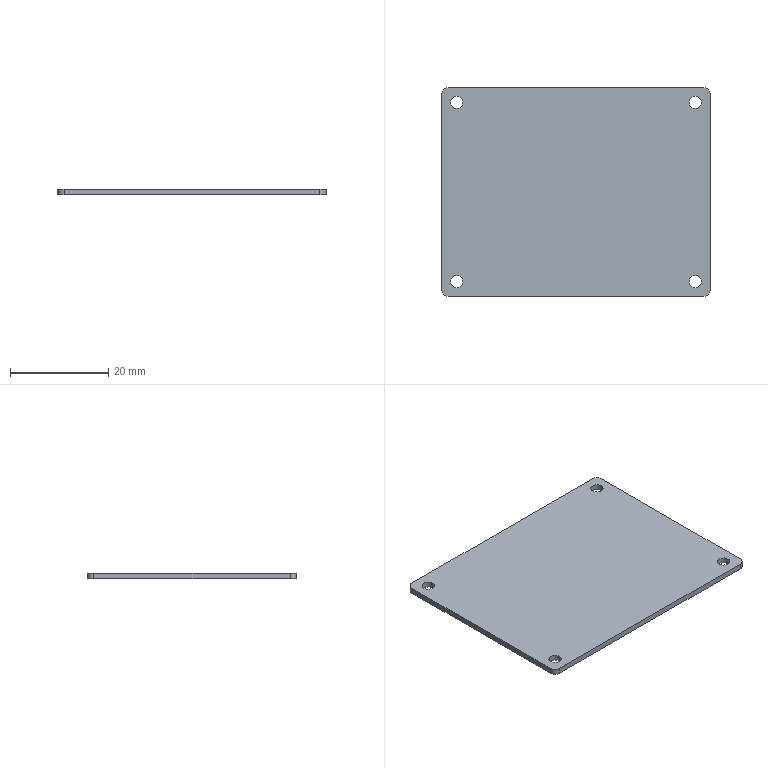Part | STEP file | Control module MCU PCB | 1 solid | 14 faces | box 54.57 x 42.52 x 1.2 mm | volume 2759 mm3 | cylinder 8 | plane 6 | commonest cylinder face diameters 2.5 x4 2.54 x4
STEP:
#1=CARTESIAN_POINT('',(0.,0.,0.));
#2=DIRECTION('',(0.,0.,1.));
#3=DIRECTION('',(1.,0.,0.));
#4=AXIS2_PLACEMENT_3D('',#1,#2,#3);
#5=CARTESIAN_POINT('',(0.209,41.243,0.));
#6=VERTEX_POINT('',#5);
#7=CARTESIAN_POINT('',(0.209,1.263,0.));
#8=VERTEX_POINT('',#7);
#9=CARTESIAN_POINT('',(0.209,41.243,0.));
#10=DIRECTION('',(0.,-1.,0.));
#11=VECTOR('',#10,1.);
#12=LINE('',#9,#11);
#13=CARTESIAN_POINT('',(0.209,41.243,-1.2));
#14=DIRECTION('',(-1.,0.,0.));
#15=DIRECTION('',(0.,0.,1.));
#16=AXIS2_PLACEMENT_3D('',#13,#14,#15);
#17=PLANE('',#16);
#18=CARTESIAN_POINT('',(1.2,0.));
#19=DIRECTION('',(0.,-1.));
#20=VECTOR('',#19,1.);
#21=LINE('',#18,#20);
#22=(GEOMETRIC_REPRESENTATION_CONTEXT(2)PARAMETRIC_REPRESENTATION_CONTEXT()REPRESENTATION_CONTEXT('',''));
#23=DEFINITIONAL_REPRESENTATION('',(#21),#22);
#24=PCURVE('',#17,#23);
#25=CARTESIAN_POINT('',(1.479,1.263,0.));
#26=DIRECTION('',(0.,0.,1.));
#27=DIRECTION('',(1.,0.,0.));
#28=AXIS2_PLACEMENT_3D('',#25,#26,#27);
#29=PLANE('',#28);
#30=CARTESIAN_POINT('',(-1.27,39.98));
#31=DIRECTION('',(0.,-1.));
#32=VECTOR('',#31,1.);
#33=LINE('',#30,#32);
#34=(GEOMETRIC_REPRESENTATION_CONTEXT(2)PARAMETRIC_REPRESENTATION_CONTEXT()REPRESENTATION_CONTEXT('',''));
#35=DEFINITIONAL_REPRESENTATION('',(#33),#34);
#36=PCURVE('',#29,#35);
#37=SURFACE_CURVE('',#12,(#24,#36),.PCURVE_S1.);
#38=EDGE_CURVE('',#6,#8,#37,.T.);
#39=ORIENTED_EDGE('',*,*,#38,.F.);
#40=CARTESIAN_POINT('',(0.209,41.243,-1.2));
#41=VERTEX_POINT('',#40);
#42=CARTESIAN_POINT('',(0.209,41.243,-1.2));
#43=DIRECTION('',(0.,0.,1.));
#44=VECTOR('',#43,1.);
#45=LINE('',#42,#44);
#46=CARTESIAN_POINT('',(0.,0.));
#47=DIRECTION('',(1.,0.));
#48=VECTOR('',#47,1.);
#49=LINE('',#46,#48);
#50=(GEOMETRIC_REPRESENTATION_CONTEXT(2)PARAMETRIC_REPRESENTATION_CONTEXT()REPRESENTATION_CONTEXT('',''));
#51=DEFINITIONAL_REPRESENTATION('',(#49),#50);
#52=PCURVE('',#17,#51);
#53=CARTESIAN_POINT('',(1.479,41.243,-1.2));
#54=DIRECTION('',(0.,0.,1.));
#55=DIRECTION('',(1.,0.,0.));
#56=AXIS2_PLACEMENT_3D('',#53,#54,#55);
#57=CYLINDRICAL_SURFACE('',#56,1.27);
#58=CARTESIAN_POINT('',(3.142,0.));
#59=DIRECTION('',(0.,1.));
#60=VECTOR('',#59,1.);
#61=LINE('',#58,#60);
#62=(GEOMETRIC_REPRESENTATION_CONTEXT(2)PARAMETRIC_REPRESENTATION_CONTEXT()REPRESENTATION_CONTEXT('',''));
#63=DEFINITIONAL_REPRESENTATION('',(#61),#62);
#64=PCURVE('',#57,#63);
#65=SURFACE_CURVE('',#45,(#52,#64),.PCURVE_S1.);
#66=EDGE_CURVE('',#41,#6,#65,.T.);
#67=ORIENTED_EDGE('',*,*,#66,.F.);
#68=CARTESIAN_POINT('',(0.209,1.263,-1.2));
#69=VERTEX_POINT('',#68);
#70=CARTESIAN_POINT('',(0.209,41.243,-1.2));
#71=DIRECTION('',(0.,-1.,0.));
#72=VECTOR('',#71,1.);
#73=LINE('',#70,#72);
#74=CARTESIAN_POINT('',(0.,0.));
#75=DIRECTION('',(0.,-1.));
#76=VECTOR('',#75,1.);
#77=LINE('',#74,#76);
#78=(GEOMETRIC_REPRESENTATION_CONTEXT(2)PARAMETRIC_REPRESENTATION_CONTEXT()REPRESENTATION_CONTEXT('',''));
#79=DEFINITIONAL_REPRESENTATION('',(#77),#78);
#80=PCURVE('',#17,#79);
#81=CARTESIAN_POINT('',(1.479,1.263,-1.2));
#82=DIRECTION('',(0.,0.,1.));
#83=DIRECTION('',(1.,0.,0.));
#84=AXIS2_PLACEMENT_3D('',#81,#82,#83);
#85=PLANE('',#84);
#86=CARTESIAN_POINT('',(-1.27,39.98));
#87=DIRECTION('',(0.,-1.));
#88=VECTOR('',#87,1.);
#89=LINE('',#86,#88);
#90=(GEOMETRIC_REPRESENTATION_CONTEXT(2)PARAMETRIC_REPRESENTATION_CONTEXT()REPRESENTATION_CONTEXT('',''));
#91=DEFINITIONAL_REPRESENTATION('',(#89),#90);
#92=PCURVE('',#85,#91);
#93=SURFACE_CURVE('',#73,(#80,#92),.PCURVE_S1.);
#94=EDGE_CURVE('',#41,#69,#93,.T.);
#95=ORIENTED_EDGE('',*,*,#94,.T.);
#96=CARTESIAN_POINT('',(0.209,1.263,-1.2));
#97=DIRECTION('',(0.,0.,1.));
#98=VECTOR('',#97,1.);
#99=LINE('',#96,#98);
#100=CARTESIAN_POINT('',(0.,-39.98));
#101=DIRECTION('',(1.,0.));
#102=VECTOR('',#101,1.);
#103=LINE('',#100,#102);
#104=(GEOMETRIC_REPRESENTATION_CONTEXT(2)PARAMETRIC_REPRESENTATION_CONTEXT()REPRESENTATION_CONTEXT('',''));
#105=DEFINITIONAL_REPRESENTATION('',(#103),#104);
#106=PCURVE('',#17,#105);
#107=CARTESIAN_POINT('',(1.479,1.263,-1.2));
#108=DIRECTION('',(0.,0.,1.));
#109=DIRECTION('',(1.,0.,0.));
#110=AXIS2_PLACEMENT_3D('',#107,#108,#109);
#111=CYLINDRICAL_SURFACE('',#110,1.27);
#112=CARTESIAN_POINT('',(3.142,0.));
#113=DIRECTION('',(0.,1.));
#114=VECTOR('',#113,1.);
#115=LINE('',#112,#114);
#116=(GEOMETRIC_REPRESENTATION_CONTEXT(2)PARAMETRIC_REPRESENTATION_CONTEXT()REPRESENTATION_CONTEXT('',''));
#117=DEFINITIONAL_REPRESENTATION('',(#115),#116);
#118=PCURVE('',#111,#117);
#119=SURFACE_CURVE('',#99,(#106,#118),.PCURVE_S1.);
#120=EDGE_CURVE('',#69,#8,#119,.T.);
#121=ORIENTED_EDGE('',*,*,#120,.T.);
#122=EDGE_LOOP('',(#39,#67,#95,#121));
#123=FACE_BOUND('',#122,.T.);
#124=ADVANCED_FACE('',(#123),#17,.T.);
#125=CARTESIAN_POINT('',(1.479,-0.007191,0.));
#126=VERTEX_POINT('',#125);
#127=CARTESIAN_POINT('',(1.479,1.263,0.));
#128=DIRECTION('',(0.,0.,1.));
#129=DIRECTION('',(1.,0.,0.));
#130=AXIS2_PLACEMENT_3D('',#127,#128,#129);
#131=CIRCLE('',#130,1.27);
#132=CARTESIAN_POINT('',(0.,1.2));
#133=DIRECTION('',(1.,0.));
#134=VECTOR('',#133,1.);
#135=LINE('',#132,#134);
#136=(GEOMETRIC_REPRESENTATION_CONTEXT(2)PARAMETRIC_REPRESENTATION_CONTEXT()REPRESENTATION_CONTEXT('',''));
#137=DEFINITIONAL_REPRESENTATION('',(#135),#136);
#138=PCURVE('',#111,#137);
#139=CARTESIAN_POINT('',(0.,0.));
#140=DIRECTION('',(1.,0.));
#141=AXIS2_PLACEMENT_2D('',#139,#140);
#142=CIRCLE('',#141,1.27);
#143=(GEOMETRIC_REPRESENTATION_CONTEXT(2)PARAMETRIC_REPRESENTATION_CONTEXT()REPRESENTATION_CONTEXT('',''));
#144=DEFINITIONAL_REPRESENTATION('',(#142),#143);
#145=PCURVE('',#29,#144);
#146=SURFACE_CURVE('',#131,(#138,#145),.PCURVE_S1.);
#147=EDGE_CURVE('',#8,#126,#146,.T.);
#148=ORIENTED_EDGE('',*,*,#147,.F.);
#149=ORIENTED_EDGE('',*,*,#120,.F.);
#150=CARTESIAN_POINT('',(1.479,-0.007191,-1.2));
#151=VERTEX_POINT('',#150);
#152=CARTESIAN_POINT('',(1.479,1.263,-1.2));
#153=DIRECTION('',(0.,0.,1.));
#154=DIRECTION('',(1.,0.,0.));
#155=AXIS2_PLACEMENT_3D('',#152,#153,#154);
#156=CIRCLE('',#155,1.27);
#157=CARTESIAN_POINT('',(0.,0.));
#158=DIRECTION('',(1.,0.));
#159=VECTOR('',#158,1.);
#160=LINE('',#157,#159);
#161=(GEOMETRIC_REPRESENTATION_CONTEXT(2)PARAMETRIC_REPRESENTATION_CONTEXT()REPRESENTATION_CONTEXT('',''));
#162=DEFINITIONAL_REPRESENTATION('',(#160),#161);
#163=PCURVE('',#111,#162);
#164=CARTESIAN_POINT('',(0.,0.));
#165=DIRECTION('',(1.,0.));
#166=AXIS2_PLACEMENT_2D('',#164,#165);
#167=CIRCLE('',#166,1.27);
#168=(GEOMETRIC_REPRESENTATION_CONTEXT(2)PARAMETRIC_REPRESENTATION_CONTEXT()REPRESENTATION_CONTEXT('',''));
#169=DEFINITIONAL_REPRESENTATION('',(#167),#168);
#170=PCURVE('',#85,#169);
#171=SURFACE_CURVE('',#156,(#163,#170),.PCURVE_S1.);
#172=EDGE_CURVE('',#69,#151,#171,.T.);
#173=ORIENTED_EDGE('',*,*,#172,.T.);
#174=CARTESIAN_POINT('',(1.479,-0.007191,-1.2));
#175=DIRECTION('',(0.,0.,1.));
#176=VECTOR('',#175,1.);
#177=LINE('',#174,#176);
#178=CARTESIAN_POINT('',(4.712,0.));
#179=DIRECTION('',(0.,1.));
#180=VECTOR('',#179,1.);
#181=LINE('',#178,#180);
#182=(GEOMETRIC_REPRESENTATION_CONTEXT(2)PARAMETRIC_REPRESENTATION_CONTEXT()REPRESENTATION_CONTEXT('',''));
#183=DEFINITIONAL_REPRESENTATION('',(#181),#182);
#184=PCURVE('',#111,#183);
#185=CARTESIAN_POINT('',(1.479,-0.007191,-1.2));
#186=DIRECTION('',(0.,-1.,0.));
#187=DIRECTION('',(0.,0.,-1.));
#188=AXIS2_PLACEMENT_3D('',#185,#186,#187);
#189=PLANE('',#188);
#190=CARTESIAN_POINT('',(0.,0.));
#191=DIRECTION('',(-1.,0.));
#192=VECTOR('',#191,1.);
#193=LINE('',#190,#192);
#194=(GEOMETRIC_REPRESENTATION_CONTEXT(2)PARAMETRIC_REPRESENTATION_CONTEXT()REPRESENTATION_CONTEXT('',''));
#195=DEFINITIONAL_REPRESENTATION('',(#193),#194);
#196=PCURVE('',#189,#195);
#197=SURFACE_CURVE('',#177,(#184,#196),.PCURVE_S1.);
#198=EDGE_CURVE('',#151,#126,#197,.T.);
#199=ORIENTED_EDGE('',*,*,#198,.T.);
#200=EDGE_LOOP('',(#148,#149,#173,#199));
#201=FACE_BOUND('',#200,.T.);
#202=ADVANCED_FACE('',(#201),#111,.T.);
#203=CARTESIAN_POINT('',(53.509,-0.007191,0.));
#204=VERTEX_POINT('',#203);
#205=CARTESIAN_POINT('',(1.479,-0.007191,0.));
#206=DIRECTION('',(1.,0.,0.));
#207=VECTOR('',#206,1.);
#208=LINE('',#205,#207);
#209=CARTESIAN_POINT('',(-1.2,0.));
#210=DIRECTION('',(0.,1.));
#211=VECTOR('',#210,1.);
#212=LINE('',#209,#211);
#213=(GEOMETRIC_REPRESENTATION_CONTEXT(2)PARAMETRIC_REPRESENTATION_CONTEXT()REPRESENTATION_CONTEXT('',''));
#214=DEFINITIONAL_REPRESENTATION('',(#212),#213);
#215=PCURVE('',#189,#214);
#216=CARTESIAN_POINT('',(0.,-1.27));
#217=DIRECTION('',(1.,0.));
#218=VECTOR('',#217,1.);
#219=LINE('',#216,#218);
#220=(GEOMETRIC_REPRESENTATION_CONTEXT(2)PARAMETRIC_REPRESENTATION_CONTEXT()REPRESENTATION_CONTEXT('',''));
#221=DEFINITIONAL_REPRESENTATION('',(#219),#220);
#222=PCURVE('',#29,#221);
#223=SURFACE_CURVE('',#208,(#215,#222),.PCURVE_S1.);
#224=EDGE_CURVE('',#126,#204,#223,.T.);
#225=ORIENTED_EDGE('',*,*,#224,.F.);
#226=ORIENTED_EDGE('',*,*,#198,.F.);
#227=CARTESIAN_POINT('',(53.509,-0.007191,-1.2));
#228=VERTEX_POINT('',#227);
#229=CARTESIAN_POINT('',(1.479,-0.007191,-1.2));
#230=DIRECTION('',(1.,0.,0.));
#231=VECTOR('',#230,1.);
#232=LINE('',#229,#231);
#233=CARTESIAN_POINT('',(0.,0.));
#234=DIRECTION('',(0.,1.));
#235=VECTOR('',#234,1.);
#236=LINE('',#233,#235);
#237=(GEOMETRIC_REPRESENTATION_CONTEXT(2)PARAMETRIC_REPRESENTATION_CONTEXT()REPRESENTATION_CONTEXT('',''));
#238=DEFINITIONAL_REPRESENTATION('',(#236),#237);
#239=PCURVE('',#189,#238);
#240=CARTESIAN_POINT('',(0.,-1.27));
#241=DIRECTION('',(1.,0.));
#242=VECTOR('',#241,1.);
#243=LINE('',#240,#242);
#244=(GEOMETRIC_REPRESENTATION_CONTEXT(2)PARAMETRIC_REPRESENTATION_CONTEXT()REPRESENTATION_CONTEXT('',''));
#245=DEFINITIONAL_REPRESENTATION('',(#243),#244);
#246=PCURVE('',#85,#245);
#247=SURFACE_CURVE('',#232,(#239,#246),.PCURVE_S1.);
#248=EDGE_CURVE('',#151,#228,#247,.T.);
#249=ORIENTED_EDGE('',*,*,#248,.T.);
#250=CARTESIAN_POINT('',(53.509,-0.007191,-1.2));
#251=DIRECTION('',(0.,0.,1.));
#252=VECTOR('',#251,1.);
#253=LINE('',#250,#252);
#254=CARTESIAN_POINT('',(0.,52.03));
#255=DIRECTION('',(-1.,0.));
#256=VECTOR('',#255,1.);
#257=LINE('',#254,#256);
#258=(GEOMETRIC_REPRESENTATION_CONTEXT(2)PARAMETRIC_REPRESENTATION_CONTEXT()REPRESENTATION_CONTEXT('',''));
#259=DEFINITIONAL_REPRESENTATION('',(#257),#258);
#260=PCURVE('',#189,#259);
#261=CARTESIAN_POINT('',(53.509,1.263,-1.2));
#262=DIRECTION('',(0.,0.,1.));
#263=DIRECTION('',(1.,0.,0.));
#264=AXIS2_PLACEMENT_3D('',#261,#262,#263);
#265=CYLINDRICAL_SURFACE('',#264,1.27);
#266=CARTESIAN_POINT('',(4.712,0.));
#267=DIRECTION('',(0.,1.));
#268=VECTOR('',#267,1.);
#269=LINE('',#266,#268);
#270=(GEOMETRIC_REPRESENTATION_CONTEXT(2)PARAMETRIC_REPRESENTATION_CONTEXT()REPRESENTATION_CONTEXT('',''));
#271=DEFINITIONAL_REPRESENTATION('',(#269),#270);
#272=PCURVE('',#265,#271);
#273=SURFACE_CURVE('',#253,(#260,#272),.PCURVE_S1.);
#274=EDGE_CURVE('',#228,#204,#273,.T.);
#275=ORIENTED_EDGE('',*,*,#274,.T.);
#276=EDGE_LOOP('',(#225,#226,#249,#275));
#277=FACE_BOUND('',#276,.T.);
#278=ADVANCED_FACE('',(#277),#189,.T.);
#279=CARTESIAN_POINT('',(54.779,1.263,0.));
#280=VERTEX_POINT('',#279);
#281=CARTESIAN_POINT('',(53.509,1.263,0.));
#282=DIRECTION('',(0.,0.,1.));
#283=DIRECTION('',(1.,0.,0.));
#284=AXIS2_PLACEMENT_3D('',#281,#282,#283);
#285=CIRCLE('',#284,1.27);
#286=CARTESIAN_POINT('',(0.,1.2));
#287=DIRECTION('',(1.,0.));
#288=VECTOR('',#287,1.);
#289=LINE('',#286,#288);
#290=(GEOMETRIC_REPRESENTATION_CONTEXT(2)PARAMETRIC_REPRESENTATION_CONTEXT()REPRESENTATION_CONTEXT('',''));
#291=DEFINITIONAL_REPRESENTATION('',(#289),#290);
#292=PCURVE('',#265,#291);
#293=CARTESIAN_POINT('',(52.03,0.));
#294=DIRECTION('',(1.,0.));
#295=AXIS2_PLACEMENT_2D('',#293,#294);
#296=CIRCLE('',#295,1.27);
#297=(GEOMETRIC_REPRESENTATION_CONTEXT(2)PARAMETRIC_REPRESENTATION_CONTEXT()REPRESENTATION_CONTEXT('',''));
#298=DEFINITIONAL_REPRESENTATION('',(#296),#297);
#299=PCURVE('',#29,#298);
#300=SURFACE_CURVE('',#285,(#292,#299),.PCURVE_S1.);
#301=EDGE_CURVE('',#204,#280,#300,.T.);
#302=ORIENTED_EDGE('',*,*,#301,.F.);
#303=ORIENTED_EDGE('',*,*,#274,.F.);
#304=CARTESIAN_POINT('',(54.779,1.263,-1.2));
#305=VERTEX_POINT('',#304);
#306=CARTESIAN_POINT('',(53.509,1.263,-1.2));
#307=DIRECTION('',(0.,0.,1.));
#308=DIRECTION('',(1.,0.,0.));
#309=AXIS2_PLACEMENT_3D('',#306,#307,#308);
#310=CIRCLE('',#309,1.27);
#311=CARTESIAN_POINT('',(0.,0.));
#312=DIRECTION('',(1.,0.));
#313=VECTOR('',#312,1.);
#314=LINE('',#311,#313);
#315=(GEOMETRIC_REPRESENTATION_CONTEXT(2)PARAMETRIC_REPRESENTATION_CONTEXT()REPRESENTATION_CONTEXT('',''));
#316=DEFINITIONAL_REPRESENTATION('',(#314),#315);
#317=PCURVE('',#265,#316);
#318=CARTESIAN_POINT('',(52.03,0.));
#319=DIRECTION('',(1.,0.));
#320=AXIS2_PLACEMENT_2D('',#318,#319);
#321=CIRCLE('',#320,1.27);
#322=(GEOMETRIC_REPRESENTATION_CONTEXT(2)PARAMETRIC_REPRESENTATION_CONTEXT()REPRESENTATION_CONTEXT('',''));
#323=DEFINITIONAL_REPRESENTATION('',(#321),#322);
#324=PCURVE('',#85,#323);
#325=SURFACE_CURVE('',#310,(#317,#324),.PCURVE_S1.);
#326=EDGE_CURVE('',#228,#305,#325,.T.);
#327=ORIENTED_EDGE('',*,*,#326,.T.);
#328=CARTESIAN_POINT('',(54.779,1.263,-1.2));
#329=DIRECTION('',(0.,0.,1.));
#330=VECTOR('',#329,1.);
#331=LINE('',#328,#330);
#332=CARTESIAN_POINT('',(6.283,0.));
#333=DIRECTION('',(0.,1.));
#334=VECTOR('',#333,1.);
#335=LINE('',#332,#334);
#336=(GEOMETRIC_REPRESENTATION_CONTEXT(2)PARAMETRIC_REPRESENTATION_CONTEXT()REPRESENTATION_CONTEXT('',''));
#337=DEFINITIONAL_REPRESENTATION('',(#335),#336);
#338=PCURVE('',#265,#337);
#339=CARTESIAN_POINT('',(54.779,1.263,-1.2));
#340=DIRECTION('',(1.,0.000000064,0.));
#341=DIRECTION('',(-0.000000064,1.,0.));
#342=AXIS2_PLACEMENT_3D('',#339,#340,#341);
#343=PLANE('',#342);
#344=CARTESIAN_POINT('',(0.,0.));
#345=DIRECTION('',(0.,1.));
#346=VECTOR('',#345,1.);
#347=LINE('',#344,#346);
#348=(GEOMETRIC_REPRESENTATION_CONTEXT(2)PARAMETRIC_REPRESENTATION_CONTEXT()REPRESENTATION_CONTEXT('',''));
#349=DEFINITIONAL_REPRESENTATION('',(#347),#348);
#350=PCURVE('',#343,#349);
#351=SURFACE_CURVE('',#331,(#338,#350),.PCURVE_S1.);
#352=EDGE_CURVE('',#305,#280,#351,.T.);
#353=ORIENTED_EDGE('',*,*,#352,.T.);
#354=EDGE_LOOP('',(#302,#303,#327,#353));
#355=FACE_BOUND('',#354,.T.);
#356=ADVANCED_FACE('',(#355),#265,.T.);
#357=CARTESIAN_POINT('',(54.779,41.243,0.));
#358=VERTEX_POINT('',#357);
#359=CARTESIAN_POINT('',(54.779,1.263,0.));
#360=DIRECTION('',(-0.000000064,1.,0.));
#361=VECTOR('',#360,1.);
#362=LINE('',#359,#361);
#363=CARTESIAN_POINT('',(0.,1.2));
#364=DIRECTION('',(1.,0.));
#365=VECTOR('',#364,1.);
#366=LINE('',#363,#365);
#367=(GEOMETRIC_REPRESENTATION_CONTEXT(2)PARAMETRIC_REPRESENTATION_CONTEXT()REPRESENTATION_CONTEXT('',''));
#368=DEFINITIONAL_REPRESENTATION('',(#366),#367);
#369=PCURVE('',#343,#368);
#370=CARTESIAN_POINT('',(53.3,0.));
#371=DIRECTION('',(-0.000000064,1.));
#372=VECTOR('',#371,1.);
#373=LINE('',#370,#372);
#374=(GEOMETRIC_REPRESENTATION_CONTEXT(2)PARAMETRIC_REPRESENTATION_CONTEXT()REPRESENTATION_CONTEXT('',''));
#375=DEFINITIONAL_REPRESENTATION('',(#373),#374);
#376=PCURVE('',#29,#375);
#377=SURFACE_CURVE('',#362,(#369,#376),.PCURVE_S1.);
#378=EDGE_CURVE('',#280,#358,#377,.T.);
#379=ORIENTED_EDGE('',*,*,#378,.F.);
#380=ORIENTED_EDGE('',*,*,#352,.F.);
#381=CARTESIAN_POINT('',(54.779,41.243,-1.2));
#382=VERTEX_POINT('',#381);
#383=CARTESIAN_POINT('',(54.779,1.263,-1.2));
#384=DIRECTION('',(-0.000000064,1.,0.));
#385=VECTOR('',#384,1.);
#386=LINE('',#383,#385);
#387=CARTESIAN_POINT('',(0.,0.));
#388=DIRECTION('',(1.,0.));
#389=VECTOR('',#388,1.);
#390=LINE('',#387,#389);
#391=(GEOMETRIC_REPRESENTATION_CONTEXT(2)PARAMETRIC_REPRESENTATION_CONTEXT()REPRESENTATION_CONTEXT('',''));
#392=DEFINITIONAL_REPRESENTATION('',(#390),#391);
#393=PCURVE('',#343,#392);
#394=CARTESIAN_POINT('',(53.3,0.));
#395=DIRECTION('',(-0.000000064,1.));
#396=VECTOR('',#395,1.);
#397=LINE('',#394,#396);
#398=(GEOMETRIC_REPRESENTATION_CONTEXT(2)PARAMETRIC_REPRESENTATION_CONTEXT()REPRESENTATION_CONTEXT('',''));
#399=DEFINITIONAL_REPRESENTATION('',(#397),#398);
#400=PCURVE('',#85,#399);
#401=SURFACE_CURVE('',#386,(#393,#400),.PCURVE_S1.);
#402=EDGE_CURVE('',#305,#382,#401,.T.);
#403=ORIENTED_EDGE('',*,*,#402,.T.);
#404=CARTESIAN_POINT('',(54.779,41.243,-1.2));
#405=DIRECTION('',(0.,0.,1.));
#406=VECTOR('',#405,1.);
#407=LINE('',#404,#406);
#408=CARTESIAN_POINT('',(39.98,0.));
#409=DIRECTION('',(0.,1.));
#410=VECTOR('',#409,1.);
#411=LINE('',#408,#410);
#412=(GEOMETRIC_REPRESENTATION_CONTEXT(2)PARAMETRIC_REPRESENTATION_CONTEXT()REPRESENTATION_CONTEXT('',''));
#413=DEFINITIONAL_REPRESENTATION('',(#411),#412);
#414=PCURVE('',#343,#413);
#415=CARTESIAN_POINT('',(53.509,41.243,-1.2));
#416=DIRECTION('',(0.,0.,1.));
#417=DIRECTION('',(1.,0.,0.));
#418=AXIS2_PLACEMENT_3D('',#415,#416,#417);
#419=CYLINDRICAL_SURFACE('',#418,1.27);
#420=CARTESIAN_POINT('',(0.,0.));
#421=DIRECTION('',(0.,1.));
#422=VECTOR('',#421,1.);
#423=LINE('',#420,#422);
#424=(GEOMETRIC_REPRESENTATION_CONTEXT(2)PARAMETRIC_REPRESENTATION_CONTEXT()REPRESENTATION_CONTEXT('',''));
#425=DEFINITIONAL_REPRESENTATION('',(#423),#424);
#426=PCURVE('',#419,#425);
#427=SURFACE_CURVE('',#407,(#414,#426),.PCURVE_S1.);
#428=EDGE_CURVE('',#382,#358,#427,.T.);
#429=ORIENTED_EDGE('',*,*,#428,.T.);
#430=EDGE_LOOP('',(#379,#380,#403,#429));
#431=FACE_BOUND('',#430,.T.);
#432=ADVANCED_FACE('',(#431),#343,.T.);
#433=CARTESIAN_POINT('',(53.509,42.513,0.));
#434=VERTEX_POINT('',#433);
#435=CARTESIAN_POINT('',(53.509,41.243,0.));
#436=DIRECTION('',(0.,0.,1.));
#437=DIRECTION('',(1.,0.,0.));
#438=AXIS2_PLACEMENT_3D('',#435,#436,#437);
#439=CIRCLE('',#438,1.27);
#440=CARTESIAN_POINT('',(0.,1.2));
#441=DIRECTION('',(1.,0.));
#442=VECTOR('',#441,1.);
#443=LINE('',#440,#442);
#444=(GEOMETRIC_REPRESENTATION_CONTEXT(2)PARAMETRIC_REPRESENTATION_CONTEXT()REPRESENTATION_CONTEXT('',''));
#445=DEFINITIONAL_REPRESENTATION('',(#443),#444);
#446=PCURVE('',#419,#445);
#447=CARTESIAN_POINT('',(52.03,39.98));
#448=DIRECTION('',(1.,0.));
#449=AXIS2_PLACEMENT_2D('',#447,#448);
#450=CIRCLE('',#449,1.27);
#451=(GEOMETRIC_REPRESENTATION_CONTEXT(2)PARAMETRIC_REPRESENTATION_CONTEXT()REPRESENTATION_CONTEXT('',''));
#452=DEFINITIONAL_REPRESENTATION('',(#450),#451);
#453=PCURVE('',#29,#452);
#454=SURFACE_CURVE('',#439,(#446,#453),.PCURVE_S1.);
#455=EDGE_CURVE('',#358,#434,#454,.T.);
#456=ORIENTED_EDGE('',*,*,#455,.F.);
#457=ORIENTED_EDGE('',*,*,#428,.F.);
#458=CARTESIAN_POINT('',(53.509,42.513,-1.2));
#459=VERTEX_POINT('',#458);
#460=CARTESIAN_POINT('',(53.509,41.243,-1.2));
#461=DIRECTION('',(0.,0.,1.));
#462=DIRECTION('',(1.,0.,0.));
#463=AXIS2_PLACEMENT_3D('',#460,#461,#462);
#464=CIRCLE('',#463,1.27);
#465=CARTESIAN_POINT('',(0.,0.));
#466=DIRECTION('',(1.,0.));
#467=VECTOR('',#466,1.);
#468=LINE('',#465,#467);
#469=(GEOMETRIC_REPRESENTATION_CONTEXT(2)PARAMETRIC_REPRESENTATION_CONTEXT()REPRESENTATION_CONTEXT('',''));
#470=DEFINITIONAL_REPRESENTATION('',(#468),#469);
#471=PCURVE('',#419,#470);
#472=CARTESIAN_POINT('',(52.03,39.98));
#473=DIRECTION('',(1.,0.));
#474=AXIS2_PLACEMENT_2D('',#472,#473);
#475=CIRCLE('',#474,1.27);
#476=(GEOMETRIC_REPRESENTATION_CONTEXT(2)PARAMETRIC_REPRESENTATION_CONTEXT()REPRESENTATION_CONTEXT('',''));
#477=DEFINITIONAL_REPRESENTATION('',(#475),#476);
#478=PCURVE('',#85,#477);
#479=SURFACE_CURVE('',#464,(#471,#478),.PCURVE_S1.);
#480=EDGE_CURVE('',#382,#459,#479,.T.);
#481=ORIENTED_EDGE('',*,*,#480,.T.);
#482=CARTESIAN_POINT('',(53.509,42.513,-1.2));
#483=DIRECTION('',(0.,0.,1.));
#484=VECTOR('',#483,1.);
#485=LINE('',#482,#484);
#486=CARTESIAN_POINT('',(1.571,0.));
#487=DIRECTION('',(0.,1.));
#488=VECTOR('',#487,1.);
#489=LINE('',#486,#488);
#490=(GEOMETRIC_REPRESENTATION_CONTEXT(2)PARAMETRIC_REPRESENTATION_CONTEXT()REPRESENTATION_CONTEXT('',''));
#491=DEFINITIONAL_REPRESENTATION('',(#489),#490);
#492=PCURVE('',#419,#491);
#493=CARTESIAN_POINT('',(53.509,42.513,-1.2));
#494=DIRECTION('',(0.,1.,0.));
#495=DIRECTION('',(0.,0.,1.));
#496=AXIS2_PLACEMENT_3D('',#493,#494,#495);
#497=PLANE('',#496);
#498=CARTESIAN_POINT('',(0.,0.));
#499=DIRECTION('',(1.,0.));
#500=VECTOR('',#499,1.);
#501=LINE('',#498,#500);
#502=(GEOMETRIC_REPRESENTATION_CONTEXT(2)PARAMETRIC_REPRESENTATION_CONTEXT()REPRESENTATION_CONTEXT('',''));
#503=DEFINITIONAL_REPRESENTATION('',(#501),#502);
#504=PCURVE('',#497,#503);
#505=SURFACE_CURVE('',#485,(#492,#504),.PCURVE_S1.);
#506=EDGE_CURVE('',#459,#434,#505,.T.);
#507=ORIENTED_EDGE('',*,*,#506,.T.);
#508=EDGE_LOOP('',(#456,#457,#481,#507));
#509=FACE_BOUND('',#508,.T.);
#510=ADVANCED_FACE('',(#509),#419,.T.);
#511=CARTESIAN_POINT('',(1.479,42.513,0.));
#512=VERTEX_POINT('',#511);
#513=CARTESIAN_POINT('',(53.509,42.513,0.));
#514=DIRECTION('',(-1.,0.,0.));
#515=VECTOR('',#514,1.);
#516=LINE('',#513,#515);
#517=CARTESIAN_POINT('',(1.2,0.));
#518=DIRECTION('',(0.,-1.));
#519=VECTOR('',#518,1.);
#520=LINE('',#517,#519);
#521=(GEOMETRIC_REPRESENTATION_CONTEXT(2)PARAMETRIC_REPRESENTATION_CONTEXT()REPRESENTATION_CONTEXT('',''));
#522=DEFINITIONAL_REPRESENTATION('',(#520),#521);
#523=PCURVE('',#497,#522);
#524=CARTESIAN_POINT('',(52.03,41.25));
#525=DIRECTION('',(-1.,0.));
#526=VECTOR('',#525,1.);
#527=LINE('',#524,#526);
#528=(GEOMETRIC_REPRESENTATION_CONTEXT(2)PARAMETRIC_REPRESENTATION_CONTEXT()REPRESENTATION_CONTEXT('',''));
#529=DEFINITIONAL_REPRESENTATION('',(#527),#528);
#530=PCURVE('',#29,#529);
#531=SURFACE_CURVE('',#516,(#523,#530),.PCURVE_S1.);
#532=EDGE_CURVE('',#434,#512,#531,.T.);
#533=ORIENTED_EDGE('',*,*,#532,.F.);
#534=ORIENTED_EDGE('',*,*,#506,.F.);
#535=CARTESIAN_POINT('',(1.479,42.513,-1.2));
#536=VERTEX_POINT('',#535);
#537=CARTESIAN_POINT('',(53.509,42.513,-1.2));
#538=DIRECTION('',(-1.,0.,0.));
#539=VECTOR('',#538,1.);
#540=LINE('',#537,#539);
#541=CARTESIAN_POINT('',(0.,0.));
#542=DIRECTION('',(0.,-1.));
#543=VECTOR('',#542,1.);
#544=LINE('',#541,#543);
#545=(GEOMETRIC_REPRESENTATION_CONTEXT(2)PARAMETRIC_REPRESENTATION_CONTEXT()REPRESENTATION_CONTEXT('',''));
#546=DEFINITIONAL_REPRESENTATION('',(#544),#545);
#547=PCURVE('',#497,#546);
#548=CARTESIAN_POINT('',(52.03,41.25));
#549=DIRECTION('',(-1.,0.));
#550=VECTOR('',#549,1.);
#551=LINE('',#548,#550);
#552=(GEOMETRIC_REPRESENTATION_CONTEXT(2)PARAMETRIC_REPRESENTATION_CONTEXT()REPRESENTATION_CONTEXT('',''));
#553=DEFINITIONAL_REPRESENTATION('',(#551),#552);
#554=PCURVE('',#85,#553);
#555=SURFACE_CURVE('',#540,(#547,#554),.PCURVE_S1.);
#556=EDGE_CURVE('',#459,#536,#555,.T.);
#557=ORIENTED_EDGE('',*,*,#556,.T.);
#558=CARTESIAN_POINT('',(1.479,42.513,-1.2));
#559=DIRECTION('',(0.,0.,1.));
#560=VECTOR('',#559,1.);
#561=LINE('',#558,#560);
#562=CARTESIAN_POINT('',(0.,-52.03));
#563=DIRECTION('',(1.,0.));
#564=VECTOR('',#563,1.);
#565=LINE('',#562,#564);
#566=(GEOMETRIC_REPRESENTATION_CONTEXT(2)PARAMETRIC_REPRESENTATION_CONTEXT()REPRESENTATION_CONTEXT('',''));
#567=DEFINITIONAL_REPRESENTATION('',(#565),#566);
#568=PCURVE('',#497,#567);
#569=CARTESIAN_POINT('',(1.571,0.));
#570=DIRECTION('',(0.,1.));
#571=VECTOR('',#570,1.);
#572=LINE('',#569,#571);
#573=(GEOMETRIC_REPRESENTATION_CONTEXT(2)PARAMETRIC_REPRESENTATION_CONTEXT()REPRESENTATION_CONTEXT('',''));
#574=DEFINITIONAL_REPRESENTATION('',(#572),#573);
#575=PCURVE('',#57,#574);
#576=SURFACE_CURVE('',#561,(#568,#575),.PCURVE_S1.);
#577=EDGE_CURVE('',#536,#512,#576,.T.);
#578=ORIENTED_EDGE('',*,*,#577,.T.);
#579=EDGE_LOOP('',(#533,#534,#557,#578));
#580=FACE_BOUND('',#579,.T.);
#581=ADVANCED_FACE('',(#580),#497,.T.);
#582=CARTESIAN_POINT('',(53.029,2.993,-1.2));
#583=VERTEX_POINT('',#582);
#584=CARTESIAN_POINT('',(51.779,2.993,-1.2));
#585=DIRECTION('',(0.,0.,1.));
#586=DIRECTION('',(1.,0.,0.));
#587=AXIS2_PLACEMENT_3D('',#584,#585,#586);
#588=CIRCLE('',#587,1.25);
#589=CARTESIAN_POINT('',(51.779,2.993,-1.2));
#590=DIRECTION('',(0.,0.,1.));
#591=DIRECTION('',(1.,0.,0.));
#592=AXIS2_PLACEMENT_3D('',#589,#590,#591);
#593=CYLINDRICAL_SURFACE('',#592,1.25);
#594=CARTESIAN_POINT('',(0.,0.));
#595=DIRECTION('',(1.,0.));
#596=VECTOR('',#595,1.);
#597=LINE('',#594,#596);
#598=(GEOMETRIC_REPRESENTATION_CONTEXT(2)PARAMETRIC_REPRESENTATION_CONTEXT()REPRESENTATION_CONTEXT('',''));
#599=DEFINITIONAL_REPRESENTATION('',(#597),#598);
#600=PCURVE('',#593,#599);
#601=CARTESIAN_POINT('',(50.3,1.73));
#602=DIRECTION('',(1.,0.));
#603=AXIS2_PLACEMENT_2D('',#601,#602);
#604=CIRCLE('',#603,1.25);
#605=(GEOMETRIC_REPRESENTATION_CONTEXT(2)PARAMETRIC_REPRESENTATION_CONTEXT()REPRESENTATION_CONTEXT('',''));
#606=DEFINITIONAL_REPRESENTATION('',(#604),#605);
#607=PCURVE('',#85,#606);
#608=SURFACE_CURVE('',#588,(#600,#607),.PCURVE_S1.);
#609=EDGE_CURVE('',#583,#583,#608,.T.);
#610=ORIENTED_EDGE('',*,*,#609,.T.);
#611=CARTESIAN_POINT('',(53.029,2.993,0.));
#612=VERTEX_POINT('',#611);
#613=CARTESIAN_POINT('',(53.029,2.993,-1.2));
#614=CARTESIAN_POINT('',(53.029,2.993,0.));
#615=B_SPLINE_CURVE_WITH_KNOTS('',1,(#613,#614),.UNSPECIFIED.,.F.,.F.,(2,2),(0.,1.2),.PIECEWISE_BEZIER_KNOTS.);
#616=CARTESIAN_POINT('',(6.283,0.));
#617=DIRECTION('',(0.,1.));
#618=VECTOR('',#617,1.);
#619=LINE('',#616,#618);
#620=(GEOMETRIC_REPRESENTATION_CONTEXT(2)PARAMETRIC_REPRESENTATION_CONTEXT()REPRESENTATION_CONTEXT('',''));
#621=DEFINITIONAL_REPRESENTATION('',(#619),#620);
#622=PCURVE('',#593,#621);
#623=CARTESIAN_POINT('',(0.,0.));
#624=DIRECTION('',(0.,1.));
#625=VECTOR('',#624,1.);
#626=LINE('',#623,#625);
#627=(GEOMETRIC_REPRESENTATION_CONTEXT(2)PARAMETRIC_REPRESENTATION_CONTEXT()REPRESENTATION_CONTEXT('',''));
#628=DEFINITIONAL_REPRESENTATION('',(#626),#627);
#629=PCURVE('',#593,#628);
#630=SEAM_CURVE('',#615,(#622,#629),.PCURVE_S1.);
#631=EDGE_CURVE('',#583,#612,#630,.T.);
#632=ORIENTED_EDGE('',*,*,#631,.T.);
#633=CARTESIAN_POINT('',(51.779,2.993,0.));
#634=DIRECTION('',(0.,0.,1.));
#635=DIRECTION('',(1.,0.,0.));
#636=AXIS2_PLACEMENT_3D('',#633,#634,#635);
#637=CIRCLE('',#636,1.25);
#638=CARTESIAN_POINT('',(0.,1.2));
#639=DIRECTION('',(1.,0.));
#640=VECTOR('',#639,1.);
#641=LINE('',#638,#640);
#642=(GEOMETRIC_REPRESENTATION_CONTEXT(2)PARAMETRIC_REPRESENTATION_CONTEXT()REPRESENTATION_CONTEXT('',''));
#643=DEFINITIONAL_REPRESENTATION('',(#641),#642);
#644=PCURVE('',#593,#643);
#645=CARTESIAN_POINT('',(50.3,1.73));
#646=DIRECTION('',(1.,0.));
#647=AXIS2_PLACEMENT_2D('',#645,#646);
#648=CIRCLE('',#647,1.25);
#649=(GEOMETRIC_REPRESENTATION_CONTEXT(2)PARAMETRIC_REPRESENTATION_CONTEXT()REPRESENTATION_CONTEXT('',''));
#650=DEFINITIONAL_REPRESENTATION('',(#648),#649);
#651=PCURVE('',#29,#650);
#652=SURFACE_CURVE('',#637,(#644,#651),.PCURVE_S1.);
#653=EDGE_CURVE('',#612,#612,#652,.T.);
#654=ORIENTED_EDGE('',*,*,#653,.F.);
#655=ORIENTED_EDGE('',*,*,#631,.F.);
#656=EDGE_LOOP('',(#610,#632,#654,#655));
#657=FACE_BOUND('',#656,.F.);
#658=ADVANCED_FACE('',(#657),#593,.F.);
#659=CARTESIAN_POINT('',(4.459,2.993,-1.2));
#660=VERTEX_POINT('',#659);
#661=CARTESIAN_POINT('',(3.209,2.993,-1.2));
#662=DIRECTION('',(0.,0.,1.));
#663=DIRECTION('',(1.,0.,0.));
#664=AXIS2_PLACEMENT_3D('',#661,#662,#663);
#665=CIRCLE('',#664,1.25);
#666=CARTESIAN_POINT('',(3.209,2.993,-1.2));
#667=DIRECTION('',(0.,0.,1.));
#668=DIRECTION('',(1.,0.,0.));
#669=AXIS2_PLACEMENT_3D('',#666,#667,#668);
#670=CYLINDRICAL_SURFACE('',#669,1.25);
#671=CARTESIAN_POINT('',(0.,0.));
#672=DIRECTION('',(1.,0.));
#673=VECTOR('',#672,1.);
#674=LINE('',#671,#673);
#675=(GEOMETRIC_REPRESENTATION_CONTEXT(2)PARAMETRIC_REPRESENTATION_CONTEXT()REPRESENTATION_CONTEXT('',''));
#676=DEFINITIONAL_REPRESENTATION('',(#674),#675);
#677=PCURVE('',#670,#676);
#678=CARTESIAN_POINT('',(1.73,1.73));
#679=DIRECTION('',(1.,0.));
#680=AXIS2_PLACEMENT_2D('',#678,#679);
#681=CIRCLE('',#680,1.25);
#682=(GEOMETRIC_REPRESENTATION_CONTEXT(2)PARAMETRIC_REPRESENTATION_CONTEXT()REPRESENTATION_CONTEXT('',''));
#683=DEFINITIONAL_REPRESENTATION('',(#681),#682);
#684=PCURVE('',#85,#683);
#685=SURFACE_CURVE('',#665,(#677,#684),.PCURVE_S1.);
#686=EDGE_CURVE('',#660,#660,#685,.T.);
#687=ORIENTED_EDGE('',*,*,#686,.T.);
#688=CARTESIAN_POINT('',(4.459,2.993,0.));
#689=VERTEX_POINT('',#688);
#690=CARTESIAN_POINT('',(4.459,2.993,-1.2));
#691=CARTESIAN_POINT('',(4.459,2.993,0.));
#692=B_SPLINE_CURVE_WITH_KNOTS('',1,(#690,#691),.UNSPECIFIED.,.F.,.F.,(2,2),(0.,1.2),.PIECEWISE_BEZIER_KNOTS.);
#693=CARTESIAN_POINT('',(6.283,0.));
#694=DIRECTION('',(0.,1.));
#695=VECTOR('',#694,1.);
#696=LINE('',#693,#695);
#697=(GEOMETRIC_REPRESENTATION_CONTEXT(2)PARAMETRIC_REPRESENTATION_CONTEXT()REPRESENTATION_CONTEXT('',''));
#698=DEFINITIONAL_REPRESENTATION('',(#696),#697);
#699=PCURVE('',#670,#698);
#700=CARTESIAN_POINT('',(0.,0.));
#701=DIRECTION('',(0.,1.));
#702=VECTOR('',#701,1.);
#703=LINE('',#700,#702);
#704=(GEOMETRIC_REPRESENTATION_CONTEXT(2)PARAMETRIC_REPRESENTATION_CONTEXT()REPRESENTATION_CONTEXT('',''));
#705=DEFINITIONAL_REPRESENTATION('',(#703),#704);
#706=PCURVE('',#670,#705);
#707=SEAM_CURVE('',#692,(#699,#706),.PCURVE_S1.);
#708=EDGE_CURVE('',#660,#689,#707,.T.);
#709=ORIENTED_EDGE('',*,*,#708,.T.);
#710=CARTESIAN_POINT('',(3.209,2.993,0.));
#711=DIRECTION('',(0.,0.,1.));
#712=DIRECTION('',(1.,0.,0.));
#713=AXIS2_PLACEMENT_3D('',#710,#711,#712);
#714=CIRCLE('',#713,1.25);
#715=CARTESIAN_POINT('',(0.,1.2));
#716=DIRECTION('',(1.,0.));
#717=VECTOR('',#716,1.);
#718=LINE('',#715,#717);
#719=(GEOMETRIC_REPRESENTATION_CONTEXT(2)PARAMETRIC_REPRESENTATION_CONTEXT()REPRESENTATION_CONTEXT('',''));
#720=DEFINITIONAL_REPRESENTATION('',(#718),#719);
#721=PCURVE('',#670,#720);
#722=CARTESIAN_POINT('',(1.73,1.73));
#723=DIRECTION('',(1.,0.));
#724=AXIS2_PLACEMENT_2D('',#722,#723);
#725=CIRCLE('',#724,1.25);
#726=(GEOMETRIC_REPRESENTATION_CONTEXT(2)PARAMETRIC_REPRESENTATION_CONTEXT()REPRESENTATION_CONTEXT('',''));
#727=DEFINITIONAL_REPRESENTATION('',(#725),#726);
#728=PCURVE('',#29,#727);
#729=SURFACE_CURVE('',#714,(#721,#728),.PCURVE_S1.);
#730=EDGE_CURVE('',#689,#689,#729,.T.);
#731=ORIENTED_EDGE('',*,*,#730,.F.);
#732=ORIENTED_EDGE('',*,*,#708,.F.);
#733=EDGE_LOOP('',(#687,#709,#731,#732));
#734=FACE_BOUND('',#733,.F.);
#735=ADVANCED_FACE('',(#734),#670,.F.);
#736=CARTESIAN_POINT('',(4.459,39.513,-1.2));
#737=VERTEX_POINT('',#736);
#738=CARTESIAN_POINT('',(3.209,39.513,-1.2));
#739=DIRECTION('',(0.,0.,1.));
#740=DIRECTION('',(1.,0.,0.));
#741=AXIS2_PLACEMENT_3D('',#738,#739,#740);
#742=CIRCLE('',#741,1.25);
#743=CARTESIAN_POINT('',(3.209,39.513,-1.2));
#744=DIRECTION('',(0.,0.,1.));
#745=DIRECTION('',(1.,0.,0.));
#746=AXIS2_PLACEMENT_3D('',#743,#744,#745);
#747=CYLINDRICAL_SURFACE('',#746,1.25);
#748=CARTESIAN_POINT('',(0.,0.));
#749=DIRECTION('',(1.,0.));
#750=VECTOR('',#749,1.);
#751=LINE('',#748,#750);
#752=(GEOMETRIC_REPRESENTATION_CONTEXT(2)PARAMETRIC_REPRESENTATION_CONTEXT()REPRESENTATION_CONTEXT('',''));
#753=DEFINITIONAL_REPRESENTATION('',(#751),#752);
#754=PCURVE('',#747,#753);
#755=CARTESIAN_POINT('',(1.73,38.25));
#756=DIRECTION('',(1.,0.));
#757=AXIS2_PLACEMENT_2D('',#755,#756);
#758=CIRCLE('',#757,1.25);
#759=(GEOMETRIC_REPRESENTATION_CONTEXT(2)PARAMETRIC_REPRESENTATION_CONTEXT()REPRESENTATION_CONTEXT('',''));
#760=DEFINITIONAL_REPRESENTATION('',(#758),#759);
#761=PCURVE('',#85,#760);
#762=SURFACE_CURVE('',#742,(#754,#761),.PCURVE_S1.);
#763=EDGE_CURVE('',#737,#737,#762,.T.);
#764=ORIENTED_EDGE('',*,*,#763,.T.);
#765=CARTESIAN_POINT('',(4.459,39.513,0.));
#766=VERTEX_POINT('',#765);
#767=CARTESIAN_POINT('',(4.459,39.513,-1.2));
#768=CARTESIAN_POINT('',(4.459,39.513,0.));
#769=B_SPLINE_CURVE_WITH_KNOTS('',1,(#767,#768),.UNSPECIFIED.,.F.,.F.,(2,2),(0.,1.2),.PIECEWISE_BEZIER_KNOTS.);
#770=CARTESIAN_POINT('',(6.283,0.));
#771=DIRECTION('',(0.,1.));
#772=VECTOR('',#771,1.);
#773=LINE('',#770,#772);
#774=(GEOMETRIC_REPRESENTATION_CONTEXT(2)PARAMETRIC_REPRESENTATION_CONTEXT()REPRESENTATION_CONTEXT('',''));
#775=DEFINITIONAL_REPRESENTATION('',(#773),#774);
#776=PCURVE('',#747,#775);
#777=CARTESIAN_POINT('',(0.,0.));
#778=DIRECTION('',(0.,1.));
#779=VECTOR('',#778,1.);
#780=LINE('',#777,#779);
#781=(GEOMETRIC_REPRESENTATION_CONTEXT(2)PARAMETRIC_REPRESENTATION_CONTEXT()REPRESENTATION_CONTEXT('',''));
#782=DEFINITIONAL_REPRESENTATION('',(#780),#781);
#783=PCURVE('',#747,#782);
#784=SEAM_CURVE('',#769,(#776,#783),.PCURVE_S1.);
#785=EDGE_CURVE('',#737,#766,#784,.T.);
#786=ORIENTED_EDGE('',*,*,#785,.T.);
#787=CARTESIAN_POINT('',(3.209,39.513,0.));
#788=DIRECTION('',(0.,0.,1.));
#789=DIRECTION('',(1.,0.,0.));
#790=AXIS2_PLACEMENT_3D('',#787,#788,#789);
#791=CIRCLE('',#790,1.25);
#792=CARTESIAN_POINT('',(0.,1.2));
#793=DIRECTION('',(1.,0.));
#794=VECTOR('',#793,1.);
#795=LINE('',#792,#794);
#796=(GEOMETRIC_REPRESENTATION_CONTEXT(2)PARAMETRIC_REPRESENTATION_CONTEXT()REPRESENTATION_CONTEXT('',''));
#797=DEFINITIONAL_REPRESENTATION('',(#795),#796);
#798=PCURVE('',#747,#797);
#799=CARTESIAN_POINT('',(1.73,38.25));
#800=DIRECTION('',(1.,0.));
#801=AXIS2_PLACEMENT_2D('',#799,#800);
#802=CIRCLE('',#801,1.25);
#803=(GEOMETRIC_REPRESENTATION_CONTEXT(2)PARAMETRIC_REPRESENTATION_CONTEXT()REPRESENTATION_CONTEXT('',''));
#804=DEFINITIONAL_REPRESENTATION('',(#802),#803);
#805=PCURVE('',#29,#804);
#806=SURFACE_CURVE('',#791,(#798,#805),.PCURVE_S1.);
#807=EDGE_CURVE('',#766,#766,#806,.T.);
#808=ORIENTED_EDGE('',*,*,#807,.F.);
#809=ORIENTED_EDGE('',*,*,#785,.F.);
#810=EDGE_LOOP('',(#764,#786,#808,#809));
#811=FACE_BOUND('',#810,.F.);
#812=ADVANCED_FACE('',(#811),#747,.F.);
#813=CARTESIAN_POINT('',(1.479,41.243,0.));
#814=DIRECTION('',(0.,0.,1.));
#815=DIRECTION('',(1.,0.,0.));
#816=AXIS2_PLACEMENT_3D('',#813,#814,#815);
#817=CIRCLE('',#816,1.27);
#818=CARTESIAN_POINT('',(0.,1.2));
#819=DIRECTION('',(1.,0.));
#820=VECTOR('',#819,1.);
#821=LINE('',#818,#820);
#822=(GEOMETRIC_REPRESENTATION_CONTEXT(2)PARAMETRIC_REPRESENTATION_CONTEXT()REPRESENTATION_CONTEXT('',''));
#823=DEFINITIONAL_REPRESENTATION('',(#821),#822);
#824=PCURVE('',#57,#823);
#825=CARTESIAN_POINT('',(0.,39.98));
#826=DIRECTION('',(1.,0.));
#827=AXIS2_PLACEMENT_2D('',#825,#826);
#828=CIRCLE('',#827,1.27);
#829=(GEOMETRIC_REPRESENTATION_CONTEXT(2)PARAMETRIC_REPRESENTATION_CONTEXT()REPRESENTATION_CONTEXT('',''));
#830=DEFINITIONAL_REPRESENTATION('',(#828),#829);
#831=PCURVE('',#29,#830);
#832=SURFACE_CURVE('',#817,(#824,#831),.PCURVE_S1.);
#833=EDGE_CURVE('',#512,#6,#832,.T.);
#834=ORIENTED_EDGE('',*,*,#833,.F.);
#835=ORIENTED_EDGE('',*,*,#577,.F.);
#836=CARTESIAN_POINT('',(1.479,41.243,-1.2));
#837=DIRECTION('',(0.,0.,1.));
#838=DIRECTION('',(1.,0.,0.));
#839=AXIS2_PLACEMENT_3D('',#836,#837,#838);
#840=CIRCLE('',#839,1.27);
#841=CARTESIAN_POINT('',(0.,0.));
#842=DIRECTION('',(1.,0.));
#843=VECTOR('',#842,1.);
#844=LINE('',#841,#843);
#845=(GEOMETRIC_REPRESENTATION_CONTEXT(2)PARAMETRIC_REPRESENTATION_CONTEXT()REPRESENTATION_CONTEXT('',''));
#846=DEFINITIONAL_REPRESENTATION('',(#844),#845);
#847=PCURVE('',#57,#846);
#848=CARTESIAN_POINT('',(0.,39.98));
#849=DIRECTION('',(1.,0.));
#850=AXIS2_PLACEMENT_2D('',#848,#849);
#851=CIRCLE('',#850,1.27);
#852=(GEOMETRIC_REPRESENTATION_CONTEXT(2)PARAMETRIC_REPRESENTATION_CONTEXT()REPRESENTATION_CONTEXT('',''));
#853=DEFINITIONAL_REPRESENTATION('',(#851),#852);
#854=PCURVE('',#85,#853);
#855=SURFACE_CURVE('',#840,(#847,#854),.PCURVE_S1.);
#856=EDGE_CURVE('',#536,#41,#855,.T.);
#857=ORIENTED_EDGE('',*,*,#856,.T.);
#858=ORIENTED_EDGE('',*,*,#66,.T.);
#859=EDGE_LOOP('',(#834,#835,#857,#858));
#860=FACE_BOUND('',#859,.T.);
#861=ADVANCED_FACE('',(#860),#57,.T.);
#862=CARTESIAN_POINT('',(53.029,39.513,-1.2));
#863=VERTEX_POINT('',#862);
#864=CARTESIAN_POINT('',(51.779,39.513,-1.2));
#865=DIRECTION('',(0.,0.,1.));
#866=DIRECTION('',(1.,0.,0.));
#867=AXIS2_PLACEMENT_3D('',#864,#865,#866);
#868=CIRCLE('',#867,1.25);
#869=CARTESIAN_POINT('',(51.779,39.513,-1.2));
#870=DIRECTION('',(0.,0.,1.));
#871=DIRECTION('',(1.,0.,0.));
#872=AXIS2_PLACEMENT_3D('',#869,#870,#871);
#873=CYLINDRICAL_SURFACE('',#872,1.25);
#874=CARTESIAN_POINT('',(0.,0.));
#875=DIRECTION('',(1.,0.));
#876=VECTOR('',#875,1.);
#877=LINE('',#874,#876);
#878=(GEOMETRIC_REPRESENTATION_CONTEXT(2)PARAMETRIC_REPRESENTATION_CONTEXT()REPRESENTATION_CONTEXT('',''));
#879=DEFINITIONAL_REPRESENTATION('',(#877),#878);
#880=PCURVE('',#873,#879);
#881=CARTESIAN_POINT('',(50.3,38.25));
#882=DIRECTION('',(1.,0.));
#883=AXIS2_PLACEMENT_2D('',#881,#882);
#884=CIRCLE('',#883,1.25);
#885=(GEOMETRIC_REPRESENTATION_CONTEXT(2)PARAMETRIC_REPRESENTATION_CONTEXT()REPRESENTATION_CONTEXT('',''));
#886=DEFINITIONAL_REPRESENTATION('',(#884),#885);
#887=PCURVE('',#85,#886);
#888=SURFACE_CURVE('',#868,(#880,#887),.PCURVE_S1.);
#889=EDGE_CURVE('',#863,#863,#888,.T.);
#890=ORIENTED_EDGE('',*,*,#889,.T.);
#891=CARTESIAN_POINT('',(53.029,39.513,0.));
#892=VERTEX_POINT('',#891);
#893=CARTESIAN_POINT('',(53.029,39.513,-1.2));
#894=CARTESIAN_POINT('',(53.029,39.513,0.));
#895=B_SPLINE_CURVE_WITH_KNOTS('',1,(#893,#894),.UNSPECIFIED.,.F.,.F.,(2,2),(0.,1.2),.PIECEWISE_BEZIER_KNOTS.);
#896=CARTESIAN_POINT('',(6.283,0.));
#897=DIRECTION('',(0.,1.));
#898=VECTOR('',#897,1.);
#899=LINE('',#896,#898);
#900=(GEOMETRIC_REPRESENTATION_CONTEXT(2)PARAMETRIC_REPRESENTATION_CONTEXT()REPRESENTATION_CONTEXT('',''));
#901=DEFINITIONAL_REPRESENTATION('',(#899),#900);
#902=PCURVE('',#873,#901);
#903=CARTESIAN_POINT('',(0.,0.));
#904=DIRECTION('',(0.,1.));
#905=VECTOR('',#904,1.);
#906=LINE('',#903,#905);
#907=(GEOMETRIC_REPRESENTATION_CONTEXT(2)PARAMETRIC_REPRESENTATION_CONTEXT()REPRESENTATION_CONTEXT('',''));
#908=DEFINITIONAL_REPRESENTATION('',(#906),#907);
#909=PCURVE('',#873,#908);
#910=SEAM_CURVE('',#895,(#902,#909),.PCURVE_S1.);
#911=EDGE_CURVE('',#863,#892,#910,.T.);
#912=ORIENTED_EDGE('',*,*,#911,.T.);
#913=CARTESIAN_POINT('',(51.779,39.513,0.));
#914=DIRECTION('',(0.,0.,1.));
#915=DIRECTION('',(1.,0.,0.));
#916=AXIS2_PLACEMENT_3D('',#913,#914,#915);
#917=CIRCLE('',#916,1.25);
#918=CARTESIAN_POINT('',(0.,1.2));
#919=DIRECTION('',(1.,0.));
#920=VECTOR('',#919,1.);
#921=LINE('',#918,#920);
#922=(GEOMETRIC_REPRESENTATION_CONTEXT(2)PARAMETRIC_REPRESENTATION_CONTEXT()REPRESENTATION_CONTEXT('',''));
#923=DEFINITIONAL_REPRESENTATION('',(#921),#922);
#924=PCURVE('',#873,#923);
#925=CARTESIAN_POINT('',(50.3,38.25));
#926=DIRECTION('',(1.,0.));
#927=AXIS2_PLACEMENT_2D('',#925,#926);
#928=CIRCLE('',#927,1.25);
#929=(GEOMETRIC_REPRESENTATION_CONTEXT(2)PARAMETRIC_REPRESENTATION_CONTEXT()REPRESENTATION_CONTEXT('',''));
#930=DEFINITIONAL_REPRESENTATION('',(#928),#929);
#931=PCURVE('',#29,#930);
#932=SURFACE_CURVE('',#917,(#924,#931),.PCURVE_S1.);
#933=EDGE_CURVE('',#892,#892,#932,.T.);
#934=ORIENTED_EDGE('',*,*,#933,.F.);
#935=ORIENTED_EDGE('',*,*,#911,.F.);
#936=EDGE_LOOP('',(#890,#912,#934,#935));
#937=FACE_BOUND('',#936,.F.);
#938=ADVANCED_FACE('',(#937),#873,.F.);
#939=ORIENTED_EDGE('',*,*,#94,.F.);
#940=ORIENTED_EDGE('',*,*,#856,.F.);
#941=ORIENTED_EDGE('',*,*,#556,.F.);
#942=ORIENTED_EDGE('',*,*,#480,.F.);
#943=ORIENTED_EDGE('',*,*,#402,.F.);
#944=ORIENTED_EDGE('',*,*,#326,.F.);
#945=ORIENTED_EDGE('',*,*,#248,.F.);
#946=ORIENTED_EDGE('',*,*,#172,.F.);
#947=EDGE_LOOP('',(#939,#940,#941,#942,#943,#944,#945,#946));
#948=FACE_BOUND('',#947,.T.);
#949=ORIENTED_EDGE('',*,*,#763,.T.);
#950=EDGE_LOOP('',(#949));
#951=FACE_BOUND('',#950,.T.);
#952=ORIENTED_EDGE('',*,*,#686,.T.);
#953=EDGE_LOOP('',(#952));
#954=FACE_BOUND('',#953,.T.);
#955=ORIENTED_EDGE('',*,*,#609,.T.);
#956=EDGE_LOOP('',(#955));
#957=FACE_BOUND('',#956,.T.);
#958=ORIENTED_EDGE('',*,*,#889,.T.);
#959=EDGE_LOOP('',(#958));
#960=FACE_BOUND('',#959,.T.);
#961=ADVANCED_FACE('',(#948,#951,#954,#957,#960),#85,.F.);
#962=ORIENTED_EDGE('',*,*,#38,.T.);
#963=ORIENTED_EDGE('',*,*,#147,.T.);
#964=ORIENTED_EDGE('',*,*,#224,.T.);
#965=ORIENTED_EDGE('',*,*,#301,.T.);
#966=ORIENTED_EDGE('',*,*,#378,.T.);
#967=ORIENTED_EDGE('',*,*,#455,.T.);
#968=ORIENTED_EDGE('',*,*,#532,.T.);
#969=ORIENTED_EDGE('',*,*,#833,.T.);
#970=EDGE_LOOP('',(#962,#963,#964,#965,#966,#967,#968,#969));
#971=FACE_BOUND('',#970,.T.);
#972=ORIENTED_EDGE('',*,*,#807,.F.);
#973=EDGE_LOOP('',(#972));
#974=FACE_BOUND('',#973,.T.);
#975=ORIENTED_EDGE('',*,*,#730,.F.);
#976=EDGE_LOOP('',(#975));
#977=FACE_BOUND('',#976,.T.);
#978=ORIENTED_EDGE('',*,*,#653,.F.);
#979=EDGE_LOOP('',(#978));
#980=FACE_BOUND('',#979,.T.);
#981=ORIENTED_EDGE('',*,*,#933,.F.);
#982=EDGE_LOOP('',(#981));
#983=FACE_BOUND('',#982,.T.);
#984=ADVANCED_FACE('',(#971,#974,#977,#980,#983),#29,.T.);
#985=CLOSED_SHELL('',(#124,#202,#278,#356,#432,#510,#581,#658,#735,#812,#861,#938,#961,#984));
#986=MANIFOLD_SOLID_BREP('',#985);
#987=(LENGTH_UNIT()NAMED_UNIT(*)SI_UNIT(.MILLI.,.METRE.));
#988=UNCERTAINTY_MEASURE_WITH_UNIT(LENGTH_MEASURE(0.000002),#987,'','');
#989=(NAMED_UNIT(*)PLANE_ANGLE_UNIT()SI_UNIT($,.RADIAN.));
#990=(NAMED_UNIT(*)SI_UNIT($,.STERADIAN.)SOLID_ANGLE_UNIT());
#991=(GEOMETRIC_REPRESENTATION_CONTEXT(3)GLOBAL_UNCERTAINTY_ASSIGNED_CONTEXT((#988))GLOBAL_UNIT_ASSIGNED_CONTEXT((#987,#989,#990))REPRESENTATION_CONTEXT('',''));
#992=ADVANCED_BREP_SHAPE_REPRESENTATION('',(#4,#986),#991);